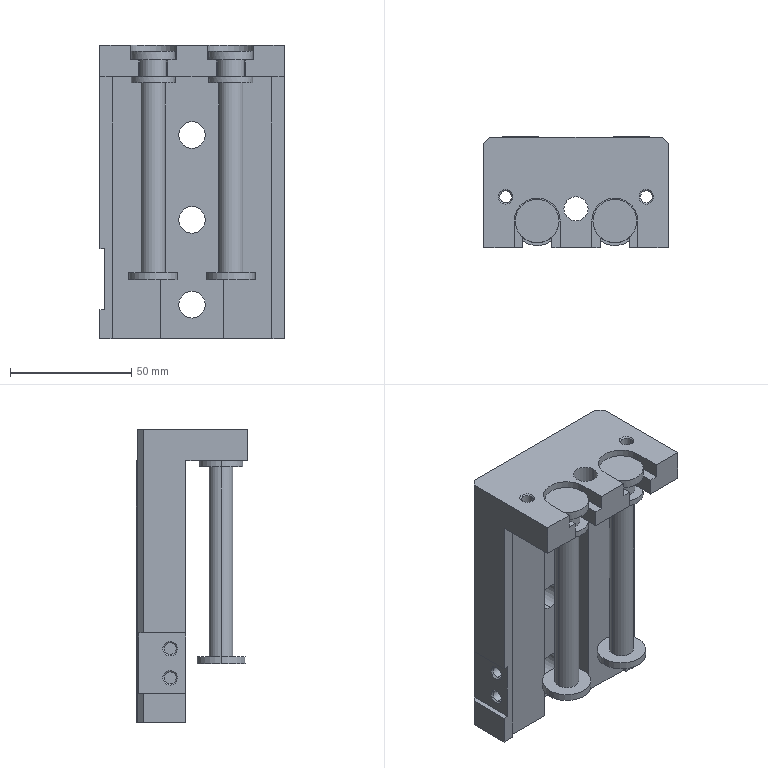Part | STEP file | _MXS20-50ASP(0)_ROD | 1 solid | 143 faces | box 76 x 46 x 121 mm | volume 178079 mm3 | plane 66 | cylinder 57 | cone 20 | commonest cylinder face diameters 4.134 x12 11 x10 4.917 x8 18 x8 10 x6 5 x5